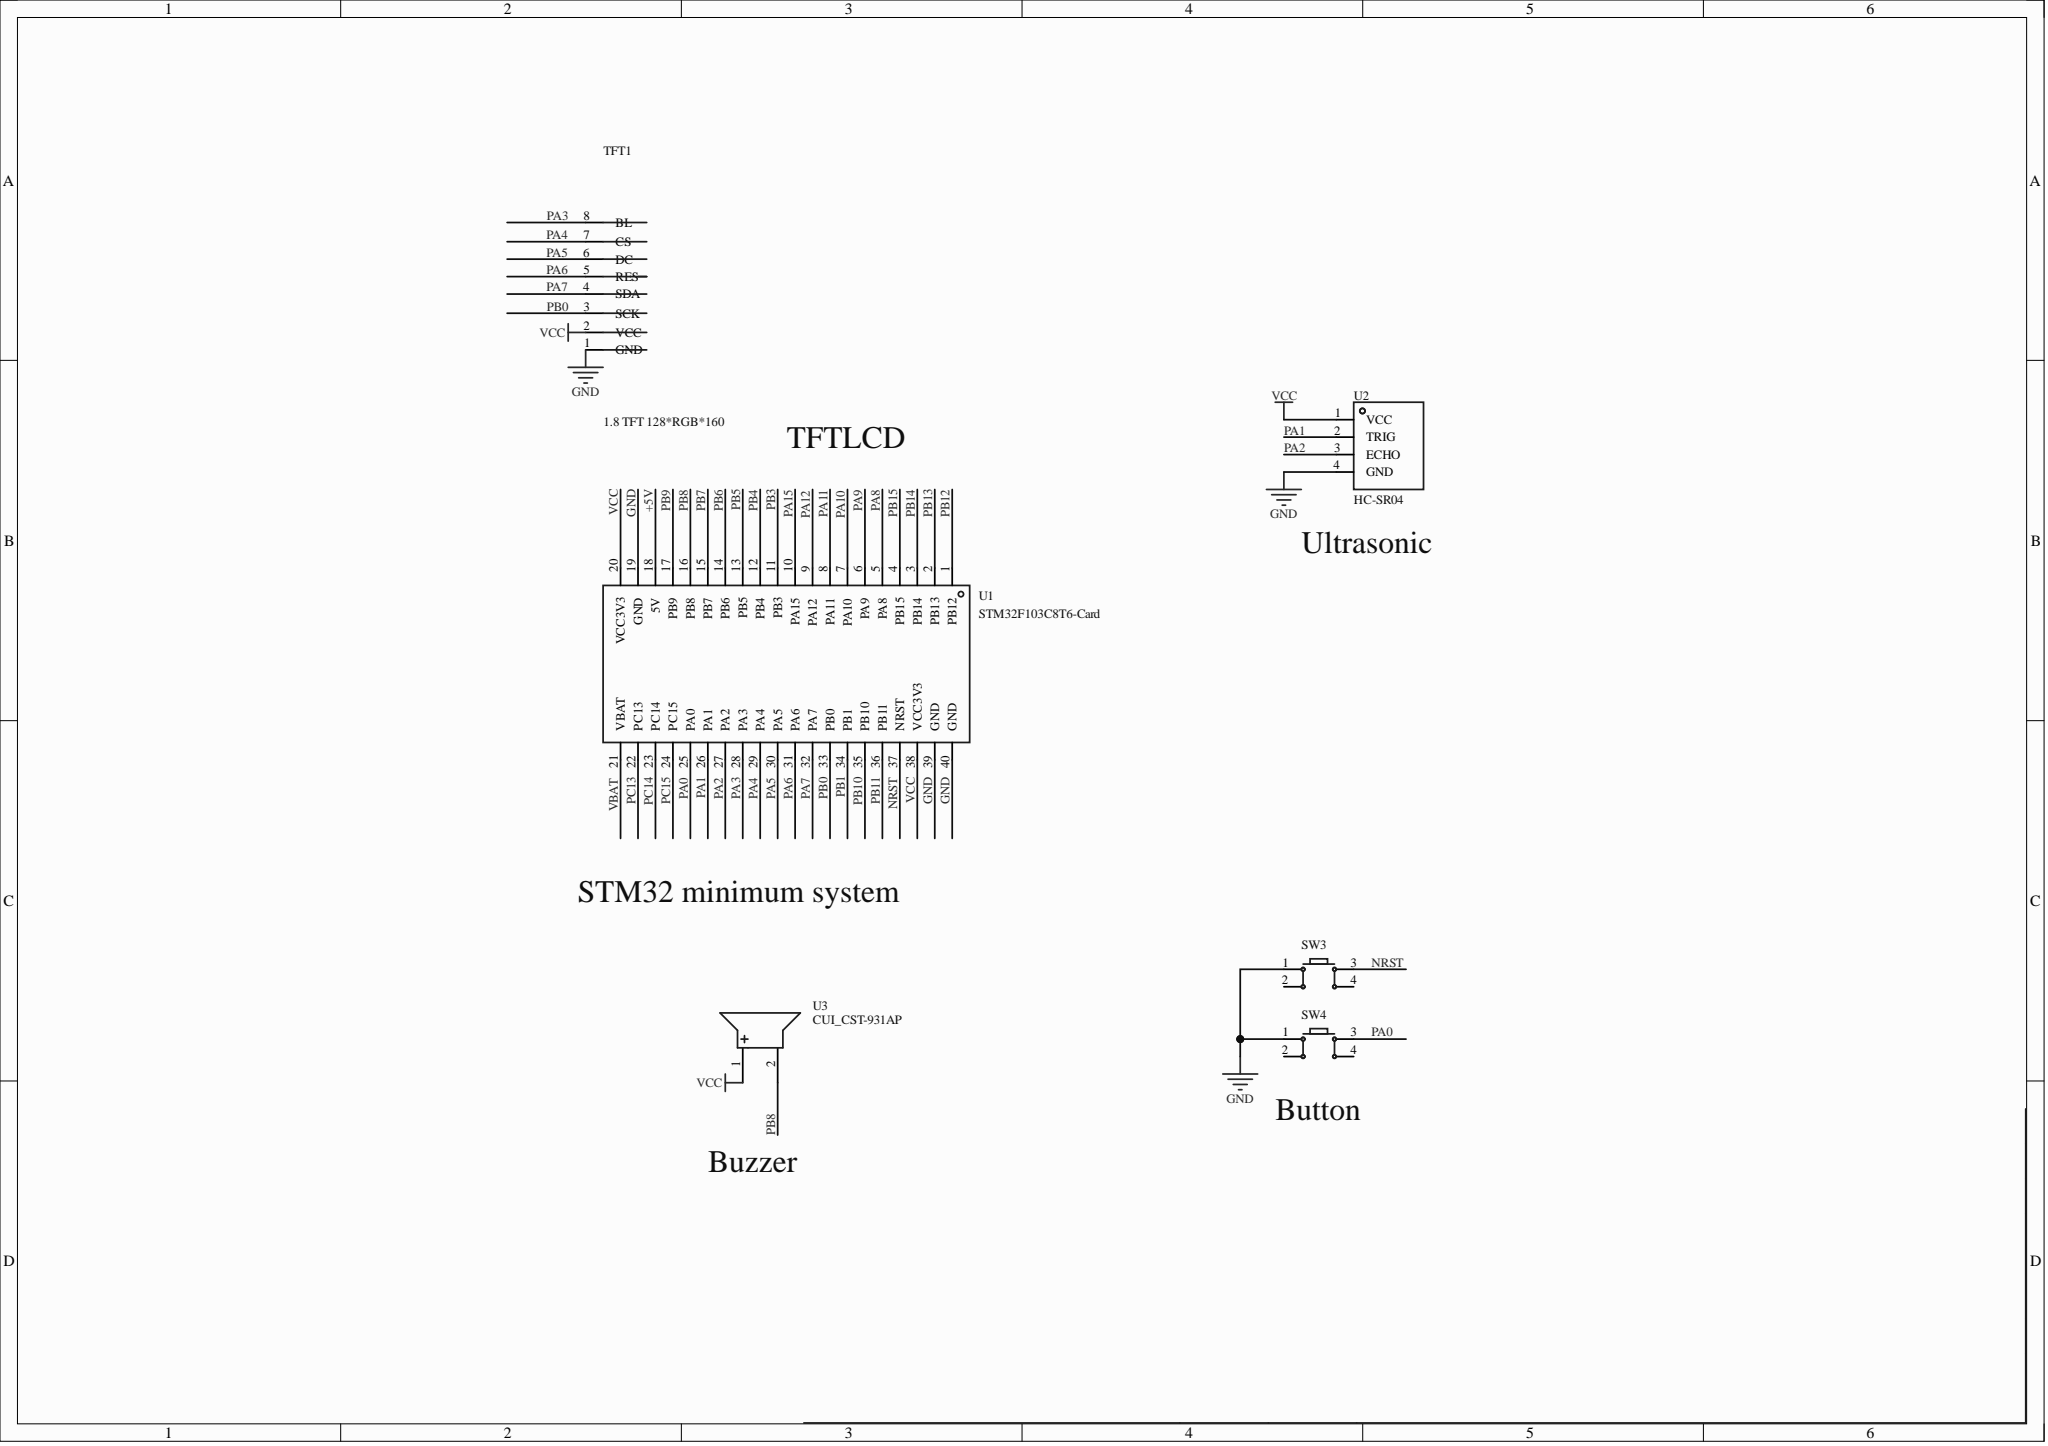Circuit board | Altium Designer | 6 parts | 13 nets
Bill of materials:
Comment,Description,Designator,Footprint,LibRef,Quantity
"","","SW3, SW4","SW-TH_4P-L6.0-W6.0-P4.50-LS6.5","Key_TH_6x6x6","2"
"1.8 TFT 128*RGB*160","","TFT1","LCD-TH_8P-P2.54-L56.0-W34.0_1.8-TFT","1.8 TFT 128*RGB*160","1"
"STM32F103C8T6-Card","","U1","CONN-TH_L53.3-W22.9_STM32F103C8T6-CARD","STM32F103C8T6-Card","1"
"HC-SR04","","U2","TH_HC-SR04V","HC-SR04","1"
"CUI_CST-931AP","","U3","BUZ-TH_BD9.0-P4.00-D0.6-L-FD","CUI_CST-931AP","1"
Netlist (Protel format):
[
SW3
SW-TH_4P-L6.0-W6.0-P4.50-LS6.5




]
[
SW4
SW-TH_4P-L6.0-W6.0-P4.50-LS6.5




]
[
TFT1
LCD-TH_8P-P2.54-L56.0-W34.0_1.8-TFT
1.8 TFT 128*RGB*160



]
[
U1
CONN-TH_L53.3-W22.9_STM32F103C8T6-CARD
STM32F103C8T6-Card



]
[
U2
TH_HC-SR04V
HC-SR04



]
[
U3
BUZ-TH_BD9.0-P4.00-D0.6-L-FD
CUI_CST-931AP



]
(
VCC
TFT1-2
U1-20
U1-38
U2-1
U3-1
)
(
PB8
U1-16
U3-2
)
(
PB0
TFT1-3
U1-33
)
(
PA7
TFT1-4
U1-32
)
(
PA6
TFT1-5
U1-31
)
(
PA5
TFT1-6
U1-30
)
(
PA4
TFT1-7
U1-29
)
(
PA3
TFT1-8
U1-28
)
(
PA2
U1-27
U2-3
)
(
PA1
U1-26
U2-2
)
(
PA0
SW4-3
U1-25
)
(
NRST
SW3-3
U1-37
)
(
GND
SW3-1
SW4-1
TFT1-1
U1-19
U1-39
U1-40
U2-4
)